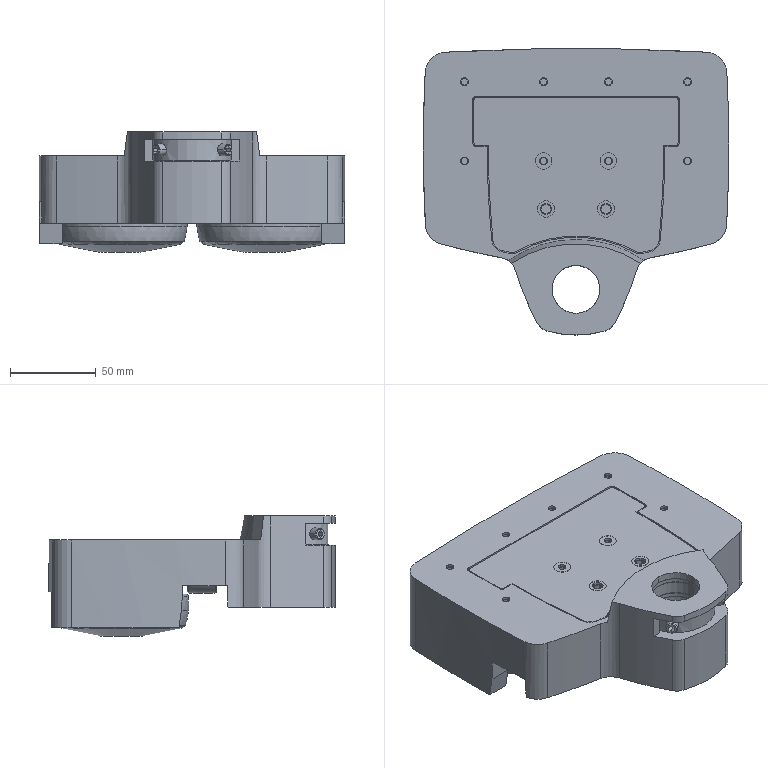Part | SolidWorks | features BaseBody 1, Scale 1 | 1 solid | 345 faces | box 178.17 x 167.027 x 70 mm | volume 882482 mm3 | plane 165 | cylinder 135 | torus 28 | cone 17 | commonest cylinder face diameters 4.55 x16 7 x16 11.2 x10 2.8 x8 9.8 x8 28 x8